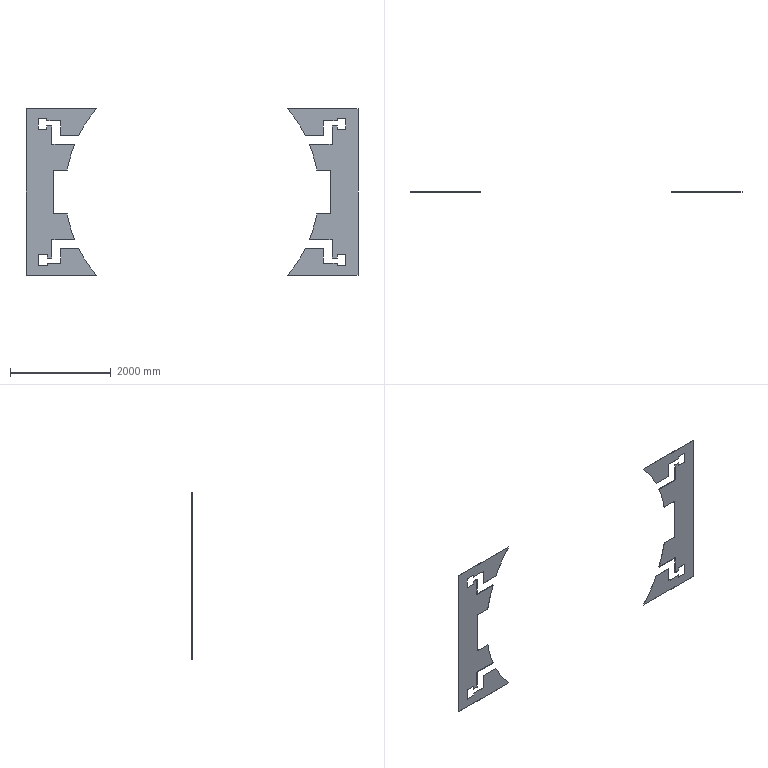Part | STEP file | Cover plate | 2 solids | 68 faces | box 6576 x 4 x 3300 mm | volume 20991561 mm3 | plane 60 | cylinder 8 | commonest cylinder face diameters 5017 x8